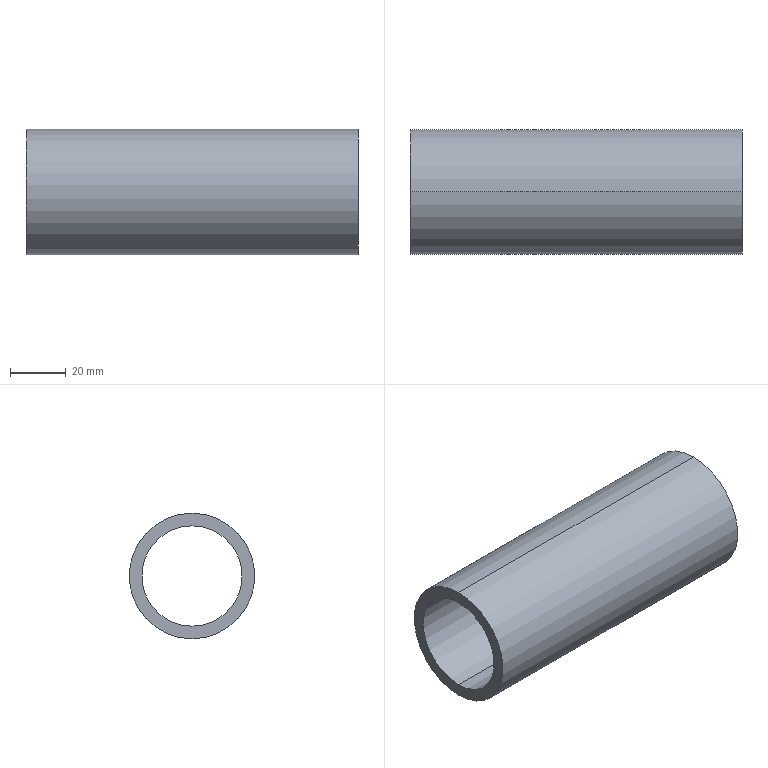Part | SolidWorks | features Extrusion 1 | 1 solid | 6 faces | box 119 x 45 x 45 mm | volume 68134 mm3 | cylinder 4 | plane 2 | commonest cylinder face diameters 36 x2 45 x2
STEP:
#1=CARTESIAN_POINT('',(119.,0.,18.));
#2=VERTEX_POINT('',#1);
#3=CARTESIAN_POINT('',(119.,0.,-18.));
#4=VERTEX_POINT('',#3);
#5=CARTESIAN_POINT('',(119.,0.,0.));
#6=DIRECTION('',(1.,0.,0.));
#7=DIRECTION('',(0.,0.,-1.));
#8=AXIS2_PLACEMENT_3D('',#5,#6,#7);
#9=CIRCLE('',#8,18.);
#10=EDGE_CURVE('',#2,#4,#9,.T.);
#11=ORIENTED_EDGE('',*,*,#10,.T.);
#12=CARTESIAN_POINT('',(0.,0.,-18.));
#13=VERTEX_POINT('',#12);
#14=CARTESIAN_POINT('',(119.,0.,-18.));
#15=DIRECTION('',(-1.,0.,0.));
#16=VECTOR('',#15,1000.);
#17=LINE('',#14,#16);
#18=EDGE_CURVE('',#4,#13,#17,.T.);
#19=ORIENTED_EDGE('',*,*,#18,.T.);
#20=CARTESIAN_POINT('',(0.,0.,18.));
#21=VERTEX_POINT('',#20);
#22=CARTESIAN_POINT('',(0.,0.,0.));
#23=DIRECTION('',(1.,0.,0.));
#24=DIRECTION('',(0.,0.,-1.));
#25=AXIS2_PLACEMENT_3D('',#22,#23,#24);
#26=CIRCLE('',#25,18.);
#27=EDGE_CURVE('',#21,#13,#26,.T.);
#28=ORIENTED_EDGE('',*,*,#27,.F.);
#29=CARTESIAN_POINT('',(119.,0.,18.));
#30=DIRECTION('',(-1.,0.,0.));
#31=VECTOR('',#30,1000.);
#32=LINE('',#29,#31);
#33=EDGE_CURVE('',#2,#21,#32,.T.);
#34=ORIENTED_EDGE('',*,*,#33,.F.);
#35=EDGE_LOOP('',(#11,#19,#28,#34));
#36=FACE_OUTER_BOUND('',#35,.T.);
#37=CARTESIAN_POINT('',(119.,0.,0.));
#38=DIRECTION('',(-1.,0.,0.));
#39=DIRECTION('',(0.,0.,1.));
#40=AXIS2_PLACEMENT_3D('',#37,#38,#39);
#41=CYLINDRICAL_SURFACE('',#40,18.);
#42=ADVANCED_FACE('',(#36),#41,.F.);
#43=CARTESIAN_POINT('',(119.,0.,-22.5));
#44=VERTEX_POINT('',#43);
#45=CARTESIAN_POINT('',(119.,0.,22.5));
#46=VERTEX_POINT('',#45);
#47=CARTESIAN_POINT('',(119.,0.,0.));
#48=DIRECTION('',(1.,0.,0.));
#49=DIRECTION('',(0.,0.,-1.));
#50=AXIS2_PLACEMENT_3D('',#47,#48,#49);
#51=CIRCLE('',#50,22.5);
#52=EDGE_CURVE('',#44,#46,#51,.T.);
#53=ORIENTED_EDGE('',*,*,#52,.F.);
#54=CARTESIAN_POINT('',(0.,0.,-22.5));
#55=VERTEX_POINT('',#54);
#56=CARTESIAN_POINT('',(119.,0.,-22.5));
#57=DIRECTION('',(-1.,0.,0.));
#58=VECTOR('',#57,1000.);
#59=LINE('',#56,#58);
#60=EDGE_CURVE('',#44,#55,#59,.T.);
#61=ORIENTED_EDGE('',*,*,#60,.T.);
#62=CARTESIAN_POINT('',(0.,0.,22.5));
#63=VERTEX_POINT('',#62);
#64=CARTESIAN_POINT('',(0.,0.,0.));
#65=DIRECTION('',(1.,0.,0.));
#66=DIRECTION('',(0.,0.,-1.));
#67=AXIS2_PLACEMENT_3D('',#64,#65,#66);
#68=CIRCLE('',#67,22.5);
#69=EDGE_CURVE('',#55,#63,#68,.T.);
#70=ORIENTED_EDGE('',*,*,#69,.T.);
#71=CARTESIAN_POINT('',(119.,0.,22.5));
#72=DIRECTION('',(-1.,0.,0.));
#73=VECTOR('',#72,1000.);
#74=LINE('',#71,#73);
#75=EDGE_CURVE('',#46,#63,#74,.T.);
#76=ORIENTED_EDGE('',*,*,#75,.F.);
#77=EDGE_LOOP('',(#53,#61,#70,#76));
#78=FACE_OUTER_BOUND('',#77,.T.);
#79=CARTESIAN_POINT('',(119.,0.,0.));
#80=DIRECTION('',(-1.,0.,0.));
#81=DIRECTION('',(0.,0.,1.));
#82=AXIS2_PLACEMENT_3D('',#79,#80,#81);
#83=CYLINDRICAL_SURFACE('',#82,22.5);
#84=ADVANCED_FACE('',(#78),#83,.T.);
#85=CARTESIAN_POINT('',(119.,0.,0.));
#86=DIRECTION('',(1.,0.,0.));
#87=DIRECTION('',(0.,0.,-1.));
#88=AXIS2_PLACEMENT_3D('',#85,#86,#87);
#89=CIRCLE('',#88,22.5);
#90=EDGE_CURVE('',#46,#44,#89,.T.);
#91=ORIENTED_EDGE('',*,*,#90,.T.);
#92=ORIENTED_EDGE('',*,*,#52,.T.);
#93=EDGE_LOOP('',(#91,#92));
#94=FACE_OUTER_BOUND('',#93,.T.);
#95=ORIENTED_EDGE('',*,*,#10,.F.);
#96=CARTESIAN_POINT('',(119.,0.,0.));
#97=DIRECTION('',(1.,0.,0.));
#98=DIRECTION('',(0.,0.,-1.));
#99=AXIS2_PLACEMENT_3D('',#96,#97,#98);
#100=CIRCLE('',#99,18.);
#101=EDGE_CURVE('',#4,#2,#100,.T.);
#102=ORIENTED_EDGE('',*,*,#101,.F.);
#103=EDGE_LOOP('',(#95,#102));
#104=FACE_BOUND('',#103,.T.);
#105=CARTESIAN_POINT('',(119.,0.,0.));
#106=DIRECTION('',(1.,0.,0.));
#107=DIRECTION('',(0.,0.,-1.));
#108=AXIS2_PLACEMENT_3D('',#105,#106,#107);
#109=PLANE('',#108);
#110=ADVANCED_FACE('',(#94,#104),#109,.T.);
#111=CARTESIAN_POINT('',(0.,0.,0.));
#112=DIRECTION('',(1.,0.,0.));
#113=DIRECTION('',(0.,0.,-1.));
#114=AXIS2_PLACEMENT_3D('',#111,#112,#113);
#115=CIRCLE('',#114,22.5);
#116=EDGE_CURVE('',#63,#55,#115,.T.);
#117=ORIENTED_EDGE('',*,*,#116,.F.);
#118=ORIENTED_EDGE('',*,*,#69,.F.);
#119=EDGE_LOOP('',(#117,#118));
#120=FACE_OUTER_BOUND('',#119,.T.);
#121=ORIENTED_EDGE('',*,*,#27,.T.);
#122=CARTESIAN_POINT('',(0.,0.,0.));
#123=DIRECTION('',(1.,0.,0.));
#124=DIRECTION('',(0.,0.,-1.));
#125=AXIS2_PLACEMENT_3D('',#122,#123,#124);
#126=CIRCLE('',#125,18.);
#127=EDGE_CURVE('',#13,#21,#126,.T.);
#128=ORIENTED_EDGE('',*,*,#127,.T.);
#129=EDGE_LOOP('',(#121,#128));
#130=FACE_BOUND('',#129,.T.);
#131=CARTESIAN_POINT('',(0.,0.,0.));
#132=DIRECTION('',(1.,0.,0.));
#133=DIRECTION('',(0.,0.,-1.));
#134=AXIS2_PLACEMENT_3D('',#131,#132,#133);
#135=PLANE('',#134);
#136=ADVANCED_FACE('',(#120,#130),#135,.F.);
#137=ORIENTED_EDGE('',*,*,#60,.F.);
#138=ORIENTED_EDGE('',*,*,#90,.F.);
#139=ORIENTED_EDGE('',*,*,#75,.T.);
#140=ORIENTED_EDGE('',*,*,#116,.T.);
#141=EDGE_LOOP('',(#137,#138,#139,#140));
#142=FACE_OUTER_BOUND('',#141,.T.);
#143=CARTESIAN_POINT('',(119.,0.,0.));
#144=DIRECTION('',(-1.,0.,0.));
#145=DIRECTION('',(0.,0.,1.));
#146=AXIS2_PLACEMENT_3D('',#143,#144,#145);
#147=CYLINDRICAL_SURFACE('',#146,22.5);
#148=ADVANCED_FACE('',(#142),#147,.T.);
#149=ORIENTED_EDGE('',*,*,#18,.F.);
#150=ORIENTED_EDGE('',*,*,#101,.T.);
#151=ORIENTED_EDGE('',*,*,#33,.T.);
#152=ORIENTED_EDGE('',*,*,#127,.F.);
#153=EDGE_LOOP('',(#149,#150,#151,#152));
#154=FACE_OUTER_BOUND('',#153,.T.);
#155=CARTESIAN_POINT('',(119.,0.,0.));
#156=DIRECTION('',(-1.,0.,0.));
#157=DIRECTION('',(0.,0.,1.));
#158=AXIS2_PLACEMENT_3D('',#155,#156,#157);
#159=CYLINDRICAL_SURFACE('',#158,18.);
#160=ADVANCED_FACE('',(#154),#159,.F.);
#161=CLOSED_SHELL('',(#42,#84,#110,#136,#148,#160));
#162=MANIFOLD_SOLID_BREP('',#161);
#163=CARTESIAN_POINT('',(0.,0.,0.));
#164=DIRECTION('',(0.,0.,1.));
#165=DIRECTION('',(1.,0.,0.));
#166=AXIS2_PLACEMENT_3D('',#163,#164,#165);
#167=(LENGTH_UNIT()NAMED_UNIT(*)SI_UNIT(.MILLI.,.METRE.));
#168=UNCERTAINTY_MEASURE_WITH_UNIT(LENGTH_MEASURE(0.00001),#167,'','');
#169=(NAMED_UNIT(*)PLANE_ANGLE_UNIT()SI_UNIT($,.RADIAN.));
#170=(NAMED_UNIT(*)SI_UNIT($,.STERADIAN.)SOLID_ANGLE_UNIT());
#171=(GEOMETRIC_REPRESENTATION_CONTEXT(3)GLOBAL_UNCERTAINTY_ASSIGNED_CONTEXT((#168))GLOBAL_UNIT_ASSIGNED_CONTEXT((#167,#169,#170))REPRESENTATION_CONTEXT('',''));
#172=ADVANCED_BREP_SHAPE_REPRESENTATION('',(#162,#166),#171);